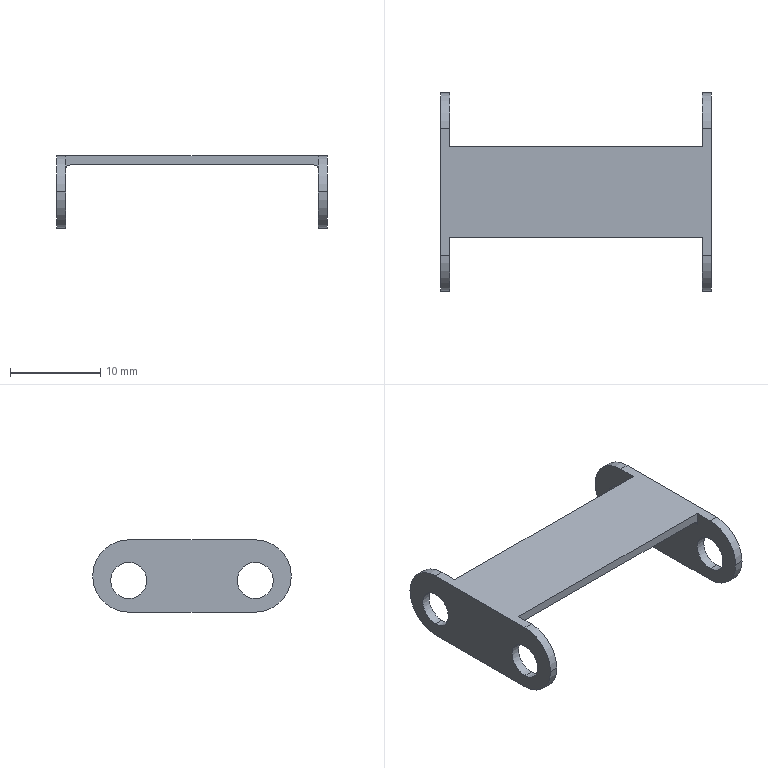Part | STEP file | Pivot Arm v2 | 1 solid | 28 faces | box 30 x 22 x 8 mm | volume 555.338 mm3 | cylinder 18 | plane 10 | commonest cylinder face diameters 4 x8 8 x8 1 x2